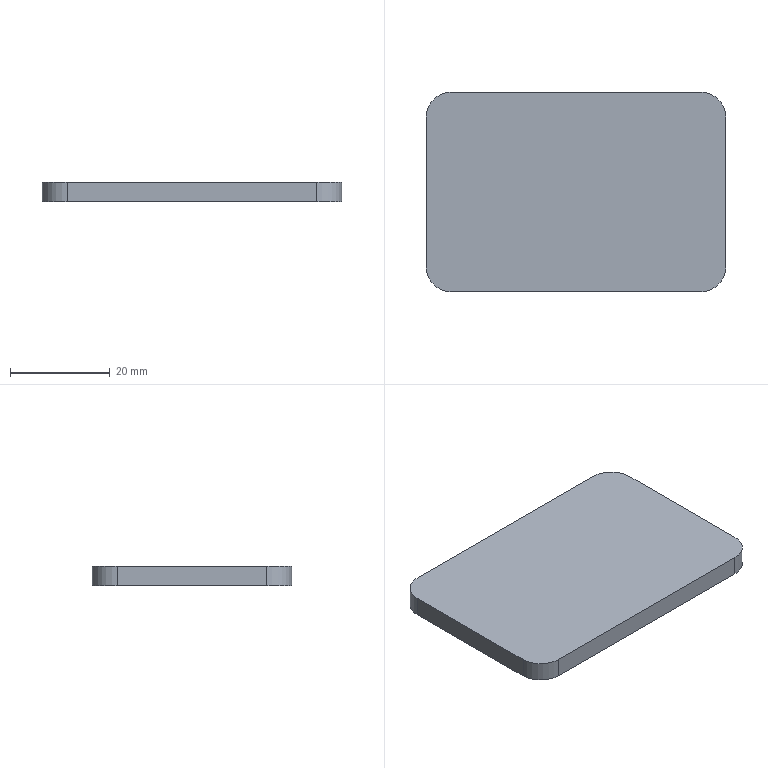Part | SolidWorks | features FlatPattern 1, SMBaseFlange 1, SheetMetal 1 | 1 solid | 10 faces | box 60 x 40 x 4 mm | volume 9514 mm3 | plane 6 | cylinder 4 | commonest cylinder face diameters 10 x4
STEP:
#1=CARTESIAN_POINT('',(-30.,-15.,0.));
#2=VERTEX_POINT('',#1);
#3=CARTESIAN_POINT('',(-25.,-20.,0.));
#4=VERTEX_POINT('',#3);
#5=CARTESIAN_POINT('',(-25.,-15.,0.));
#6=DIRECTION('',(0.,0.,1.));
#7=DIRECTION('',(1.,0.,0.));
#8=AXIS2_PLACEMENT_3D('',#5,#6,#7);
#9=CIRCLE('',#8,5.);
#10=EDGE_CURVE('',#2,#4,#9,.T.);
#11=ORIENTED_EDGE('',*,*,#10,.F.);
#12=CARTESIAN_POINT('',(-30.,-15.,-4.));
#13=VERTEX_POINT('',#12);
#14=CARTESIAN_POINT('',(-30.,-15.,-4.));
#15=DIRECTION('',(0.,0.,1.));
#16=VECTOR('',#15,1000.);
#17=LINE('',#14,#16);
#18=EDGE_CURVE('',#13,#2,#17,.T.);
#19=ORIENTED_EDGE('',*,*,#18,.F.);
#20=CARTESIAN_POINT('',(-25.,-20.,-4.));
#21=VERTEX_POINT('',#20);
#22=CARTESIAN_POINT('',(-25.,-15.,-4.));
#23=DIRECTION('',(0.,0.,1.));
#24=DIRECTION('',(1.,0.,0.));
#25=AXIS2_PLACEMENT_3D('',#22,#23,#24);
#26=CIRCLE('',#25,5.);
#27=EDGE_CURVE('',#13,#21,#26,.T.);
#28=ORIENTED_EDGE('',*,*,#27,.T.);
#29=CARTESIAN_POINT('',(-25.,-20.,-4.));
#30=DIRECTION('',(0.,0.,1.));
#31=VECTOR('',#30,1000.);
#32=LINE('',#29,#31);
#33=EDGE_CURVE('',#21,#4,#32,.T.);
#34=ORIENTED_EDGE('',*,*,#33,.T.);
#35=EDGE_LOOP('',(#11,#19,#28,#34));
#36=FACE_OUTER_BOUND('',#35,.T.);
#37=CARTESIAN_POINT('',(-25.,-15.,-4.));
#38=DIRECTION('',(0.,0.,1.));
#39=DIRECTION('',(1.,0.,0.));
#40=AXIS2_PLACEMENT_3D('',#37,#38,#39);
#41=CYLINDRICAL_SURFACE('',#40,5.);
#42=ADVANCED_FACE('',(#36),#41,.T.);
#43=CARTESIAN_POINT('',(-30.,15.,0.));
#44=VERTEX_POINT('',#43);
#45=CARTESIAN_POINT('',(-30.,15.,0.));
#46=DIRECTION('',(0.,-1.,0.));
#47=VECTOR('',#46,1000.);
#48=LINE('',#45,#47);
#49=EDGE_CURVE('',#44,#2,#48,.T.);
#50=ORIENTED_EDGE('',*,*,#49,.F.);
#51=CARTESIAN_POINT('',(-30.,15.,-4.));
#52=VERTEX_POINT('',#51);
#53=CARTESIAN_POINT('',(-30.,15.,-4.));
#54=DIRECTION('',(0.,0.,1.));
#55=VECTOR('',#54,1000.);
#56=LINE('',#53,#55);
#57=EDGE_CURVE('',#52,#44,#56,.T.);
#58=ORIENTED_EDGE('',*,*,#57,.F.);
#59=CARTESIAN_POINT('',(-30.,15.,-4.));
#60=DIRECTION('',(0.,-1.,0.));
#61=VECTOR('',#60,1000.);
#62=LINE('',#59,#61);
#63=EDGE_CURVE('',#52,#13,#62,.T.);
#64=ORIENTED_EDGE('',*,*,#63,.T.);
#65=ORIENTED_EDGE('',*,*,#18,.T.);
#66=EDGE_LOOP('',(#50,#58,#64,#65));
#67=FACE_OUTER_BOUND('',#66,.T.);
#68=CARTESIAN_POINT('',(-30.,15.,-4.));
#69=DIRECTION('',(-1.,0.,0.));
#70=DIRECTION('',(0.,-1.,0.));
#71=AXIS2_PLACEMENT_3D('',#68,#69,#70);
#72=PLANE('',#71);
#73=ADVANCED_FACE('',(#67),#72,.T.);
#74=CARTESIAN_POINT('',(-25.,20.,0.));
#75=VERTEX_POINT('',#74);
#76=CARTESIAN_POINT('',(-25.,15.,0.));
#77=DIRECTION('',(0.,0.,1.));
#78=DIRECTION('',(1.,0.,0.));
#79=AXIS2_PLACEMENT_3D('',#76,#77,#78);
#80=CIRCLE('',#79,5.);
#81=EDGE_CURVE('',#75,#44,#80,.T.);
#82=ORIENTED_EDGE('',*,*,#81,.F.);
#83=CARTESIAN_POINT('',(-25.,20.,-4.));
#84=VERTEX_POINT('',#83);
#85=CARTESIAN_POINT('',(-25.,20.,-4.));
#86=DIRECTION('',(0.,0.,1.));
#87=VECTOR('',#86,1000.);
#88=LINE('',#85,#87);
#89=EDGE_CURVE('',#84,#75,#88,.T.);
#90=ORIENTED_EDGE('',*,*,#89,.F.);
#91=CARTESIAN_POINT('',(-25.,15.,-4.));
#92=DIRECTION('',(0.,0.,1.));
#93=DIRECTION('',(1.,0.,0.));
#94=AXIS2_PLACEMENT_3D('',#91,#92,#93);
#95=CIRCLE('',#94,5.);
#96=EDGE_CURVE('',#84,#52,#95,.T.);
#97=ORIENTED_EDGE('',*,*,#96,.T.);
#98=ORIENTED_EDGE('',*,*,#57,.T.);
#99=EDGE_LOOP('',(#82,#90,#97,#98));
#100=FACE_OUTER_BOUND('',#99,.T.);
#101=CARTESIAN_POINT('',(-25.,15.,-4.));
#102=DIRECTION('',(0.,0.,1.));
#103=DIRECTION('',(1.,0.,0.));
#104=AXIS2_PLACEMENT_3D('',#101,#102,#103);
#105=CYLINDRICAL_SURFACE('',#104,5.);
#106=ADVANCED_FACE('',(#100),#105,.T.);
#107=CARTESIAN_POINT('',(25.,20.,0.));
#108=VERTEX_POINT('',#107);
#109=CARTESIAN_POINT('',(-25.,20.,0.));
#110=DIRECTION('',(-1.,0.,0.));
#111=VECTOR('',#110,1000.);
#112=LINE('',#109,#111);
#113=EDGE_CURVE('',#108,#75,#112,.T.);
#114=ORIENTED_EDGE('',*,*,#113,.F.);
#115=CARTESIAN_POINT('',(25.,20.,-4.));
#116=VERTEX_POINT('',#115);
#117=CARTESIAN_POINT('',(25.,20.,-4.));
#118=DIRECTION('',(0.,0.,1.));
#119=VECTOR('',#118,1000.);
#120=LINE('',#117,#119);
#121=EDGE_CURVE('',#116,#108,#120,.T.);
#122=ORIENTED_EDGE('',*,*,#121,.F.);
#123=CARTESIAN_POINT('',(-25.,20.,-4.));
#124=DIRECTION('',(-1.,0.,0.));
#125=VECTOR('',#124,1000.);
#126=LINE('',#123,#125);
#127=EDGE_CURVE('',#116,#84,#126,.T.);
#128=ORIENTED_EDGE('',*,*,#127,.T.);
#129=ORIENTED_EDGE('',*,*,#89,.T.);
#130=EDGE_LOOP('',(#114,#122,#128,#129));
#131=FACE_OUTER_BOUND('',#130,.T.);
#132=CARTESIAN_POINT('',(-25.,20.,-4.));
#133=DIRECTION('',(0.,1.,0.));
#134=DIRECTION('',(-1.,0.,0.));
#135=AXIS2_PLACEMENT_3D('',#132,#133,#134);
#136=PLANE('',#135);
#137=ADVANCED_FACE('',(#131),#136,.T.);
#138=CARTESIAN_POINT('',(30.,15.,0.));
#139=VERTEX_POINT('',#138);
#140=CARTESIAN_POINT('',(25.,15.,0.));
#141=DIRECTION('',(0.,0.,1.));
#142=DIRECTION('',(-1.,0.,0.));
#143=AXIS2_PLACEMENT_3D('',#140,#141,#142);
#144=CIRCLE('',#143,5.);
#145=EDGE_CURVE('',#139,#108,#144,.T.);
#146=ORIENTED_EDGE('',*,*,#145,.F.);
#147=CARTESIAN_POINT('',(30.,15.,-4.));
#148=VERTEX_POINT('',#147);
#149=CARTESIAN_POINT('',(30.,15.,-4.));
#150=DIRECTION('',(0.,0.,1.));
#151=VECTOR('',#150,1000.);
#152=LINE('',#149,#151);
#153=EDGE_CURVE('',#148,#139,#152,.T.);
#154=ORIENTED_EDGE('',*,*,#153,.F.);
#155=CARTESIAN_POINT('',(25.,15.,-4.));
#156=DIRECTION('',(0.,0.,1.));
#157=DIRECTION('',(-1.,0.,0.));
#158=AXIS2_PLACEMENT_3D('',#155,#156,#157);
#159=CIRCLE('',#158,5.);
#160=EDGE_CURVE('',#148,#116,#159,.T.);
#161=ORIENTED_EDGE('',*,*,#160,.T.);
#162=ORIENTED_EDGE('',*,*,#121,.T.);
#163=EDGE_LOOP('',(#146,#154,#161,#162));
#164=FACE_OUTER_BOUND('',#163,.T.);
#165=CARTESIAN_POINT('',(25.,15.,-4.));
#166=DIRECTION('',(0.,0.,1.));
#167=DIRECTION('',(1.,0.,0.));
#168=AXIS2_PLACEMENT_3D('',#165,#166,#167);
#169=CYLINDRICAL_SURFACE('',#168,5.);
#170=ADVANCED_FACE('',(#164),#169,.T.);
#171=CARTESIAN_POINT('',(30.,-15.,0.));
#172=VERTEX_POINT('',#171);
#173=CARTESIAN_POINT('',(30.,15.,0.));
#174=DIRECTION('',(0.,1.,0.));
#175=VECTOR('',#174,1000.);
#176=LINE('',#173,#175);
#177=EDGE_CURVE('',#172,#139,#176,.T.);
#178=ORIENTED_EDGE('',*,*,#177,.F.);
#179=CARTESIAN_POINT('',(30.,-15.,-4.));
#180=VERTEX_POINT('',#179);
#181=CARTESIAN_POINT('',(30.,-15.,-4.));
#182=DIRECTION('',(0.,0.,1.));
#183=VECTOR('',#182,1000.);
#184=LINE('',#181,#183);
#185=EDGE_CURVE('',#180,#172,#184,.T.);
#186=ORIENTED_EDGE('',*,*,#185,.F.);
#187=CARTESIAN_POINT('',(30.,15.,-4.));
#188=DIRECTION('',(0.,1.,0.));
#189=VECTOR('',#188,1000.);
#190=LINE('',#187,#189);
#191=EDGE_CURVE('',#180,#148,#190,.T.);
#192=ORIENTED_EDGE('',*,*,#191,.T.);
#193=ORIENTED_EDGE('',*,*,#153,.T.);
#194=EDGE_LOOP('',(#178,#186,#192,#193));
#195=FACE_OUTER_BOUND('',#194,.T.);
#196=CARTESIAN_POINT('',(30.,15.,-4.));
#197=DIRECTION('',(1.,0.,0.));
#198=DIRECTION('',(0.,1.,0.));
#199=AXIS2_PLACEMENT_3D('',#196,#197,#198);
#200=PLANE('',#199);
#201=ADVANCED_FACE('',(#195),#200,.T.);
#202=CARTESIAN_POINT('',(25.,-20.,0.));
#203=VERTEX_POINT('',#202);
#204=CARTESIAN_POINT('',(25.,-15.,0.));
#205=DIRECTION('',(0.,0.,1.));
#206=DIRECTION('',(1.,0.,0.));
#207=AXIS2_PLACEMENT_3D('',#204,#205,#206);
#208=CIRCLE('',#207,5.);
#209=EDGE_CURVE('',#203,#172,#208,.T.);
#210=ORIENTED_EDGE('',*,*,#209,.F.);
#211=CARTESIAN_POINT('',(25.,-20.,-4.));
#212=VERTEX_POINT('',#211);
#213=CARTESIAN_POINT('',(25.,-20.,-4.));
#214=DIRECTION('',(0.,0.,1.));
#215=VECTOR('',#214,1000.);
#216=LINE('',#213,#215);
#217=EDGE_CURVE('',#212,#203,#216,.T.);
#218=ORIENTED_EDGE('',*,*,#217,.F.);
#219=CARTESIAN_POINT('',(25.,-15.,-4.));
#220=DIRECTION('',(0.,0.,1.));
#221=DIRECTION('',(1.,0.,0.));
#222=AXIS2_PLACEMENT_3D('',#219,#220,#221);
#223=CIRCLE('',#222,5.);
#224=EDGE_CURVE('',#212,#180,#223,.T.);
#225=ORIENTED_EDGE('',*,*,#224,.T.);
#226=ORIENTED_EDGE('',*,*,#185,.T.);
#227=EDGE_LOOP('',(#210,#218,#225,#226));
#228=FACE_OUTER_BOUND('',#227,.T.);
#229=CARTESIAN_POINT('',(25.,-15.,-4.));
#230=DIRECTION('',(0.,0.,1.));
#231=DIRECTION('',(1.,0.,0.));
#232=AXIS2_PLACEMENT_3D('',#229,#230,#231);
#233=CYLINDRICAL_SURFACE('',#232,5.);
#234=ADVANCED_FACE('',(#228),#233,.T.);
#235=CARTESIAN_POINT('',(-25.,-20.,0.));
#236=DIRECTION('',(1.,0.,0.));
#237=VECTOR('',#236,1000.);
#238=LINE('',#235,#237);
#239=EDGE_CURVE('',#4,#203,#238,.T.);
#240=ORIENTED_EDGE('',*,*,#239,.F.);
#241=ORIENTED_EDGE('',*,*,#33,.F.);
#242=CARTESIAN_POINT('',(-25.,-20.,-4.));
#243=DIRECTION('',(1.,0.,0.));
#244=VECTOR('',#243,1000.);
#245=LINE('',#242,#244);
#246=EDGE_CURVE('',#21,#212,#245,.T.);
#247=ORIENTED_EDGE('',*,*,#246,.T.);
#248=ORIENTED_EDGE('',*,*,#217,.T.);
#249=EDGE_LOOP('',(#240,#241,#247,#248));
#250=FACE_OUTER_BOUND('',#249,.T.);
#251=CARTESIAN_POINT('',(-25.,-20.,-4.));
#252=DIRECTION('',(0.,-1.,0.));
#253=DIRECTION('',(0.,0.,-1.));
#254=AXIS2_PLACEMENT_3D('',#251,#252,#253);
#255=PLANE('',#254);
#256=ADVANCED_FACE('',(#250),#255,.T.);
#257=ORIENTED_EDGE('',*,*,#27,.F.);
#258=ORIENTED_EDGE('',*,*,#63,.F.);
#259=ORIENTED_EDGE('',*,*,#96,.F.);
#260=ORIENTED_EDGE('',*,*,#127,.F.);
#261=ORIENTED_EDGE('',*,*,#160,.F.);
#262=ORIENTED_EDGE('',*,*,#191,.F.);
#263=ORIENTED_EDGE('',*,*,#224,.F.);
#264=ORIENTED_EDGE('',*,*,#246,.F.);
#265=EDGE_LOOP('',(#257,#258,#259,#260,#261,#262,#263,#264));
#266=FACE_OUTER_BOUND('',#265,.T.);
#267=CARTESIAN_POINT('',(-25.,-15.,-4.));
#268=DIRECTION('',(0.,0.,1.));
#269=DIRECTION('',(1.,0.,0.));
#270=AXIS2_PLACEMENT_3D('',#267,#268,#269);
#271=PLANE('',#270);
#272=ADVANCED_FACE('',(#266),#271,.F.);
#273=ORIENTED_EDGE('',*,*,#10,.T.);
#274=ORIENTED_EDGE('',*,*,#239,.T.);
#275=ORIENTED_EDGE('',*,*,#209,.T.);
#276=ORIENTED_EDGE('',*,*,#177,.T.);
#277=ORIENTED_EDGE('',*,*,#145,.T.);
#278=ORIENTED_EDGE('',*,*,#113,.T.);
#279=ORIENTED_EDGE('',*,*,#81,.T.);
#280=ORIENTED_EDGE('',*,*,#49,.T.);
#281=EDGE_LOOP('',(#273,#274,#275,#276,#277,#278,#279,#280));
#282=FACE_OUTER_BOUND('',#281,.T.);
#283=CARTESIAN_POINT('',(-25.,-15.,0.));
#284=DIRECTION('',(0.,0.,1.));
#285=DIRECTION('',(1.,0.,0.));
#286=AXIS2_PLACEMENT_3D('',#283,#284,#285);
#287=PLANE('',#286);
#288=ADVANCED_FACE('',(#282),#287,.T.);
#289=CLOSED_SHELL('',(#42,#73,#106,#137,#170,#201,#234,#256,#272,#288));
#290=MANIFOLD_SOLID_BREP('',#289);
#291=CARTESIAN_POINT('',(0.,0.,0.));
#292=DIRECTION('',(0.,0.,1.));
#293=DIRECTION('',(1.,0.,0.));
#294=AXIS2_PLACEMENT_3D('',#291,#292,#293);
#295=(LENGTH_UNIT()NAMED_UNIT(*)SI_UNIT(.MILLI.,.METRE.));
#296=UNCERTAINTY_MEASURE_WITH_UNIT(LENGTH_MEASURE(0.00001),#295,'','');
#297=(NAMED_UNIT(*)PLANE_ANGLE_UNIT()SI_UNIT($,.RADIAN.));
#298=(NAMED_UNIT(*)SI_UNIT($,.STERADIAN.)SOLID_ANGLE_UNIT());
#299=(GEOMETRIC_REPRESENTATION_CONTEXT(3)GLOBAL_UNCERTAINTY_ASSIGNED_CONTEXT((#296))GLOBAL_UNIT_ASSIGNED_CONTEXT((#295,#297,#298))REPRESENTATION_CONTEXT('',''));
#300=ADVANCED_BREP_SHAPE_REPRESENTATION('',(#290,#294),#299);